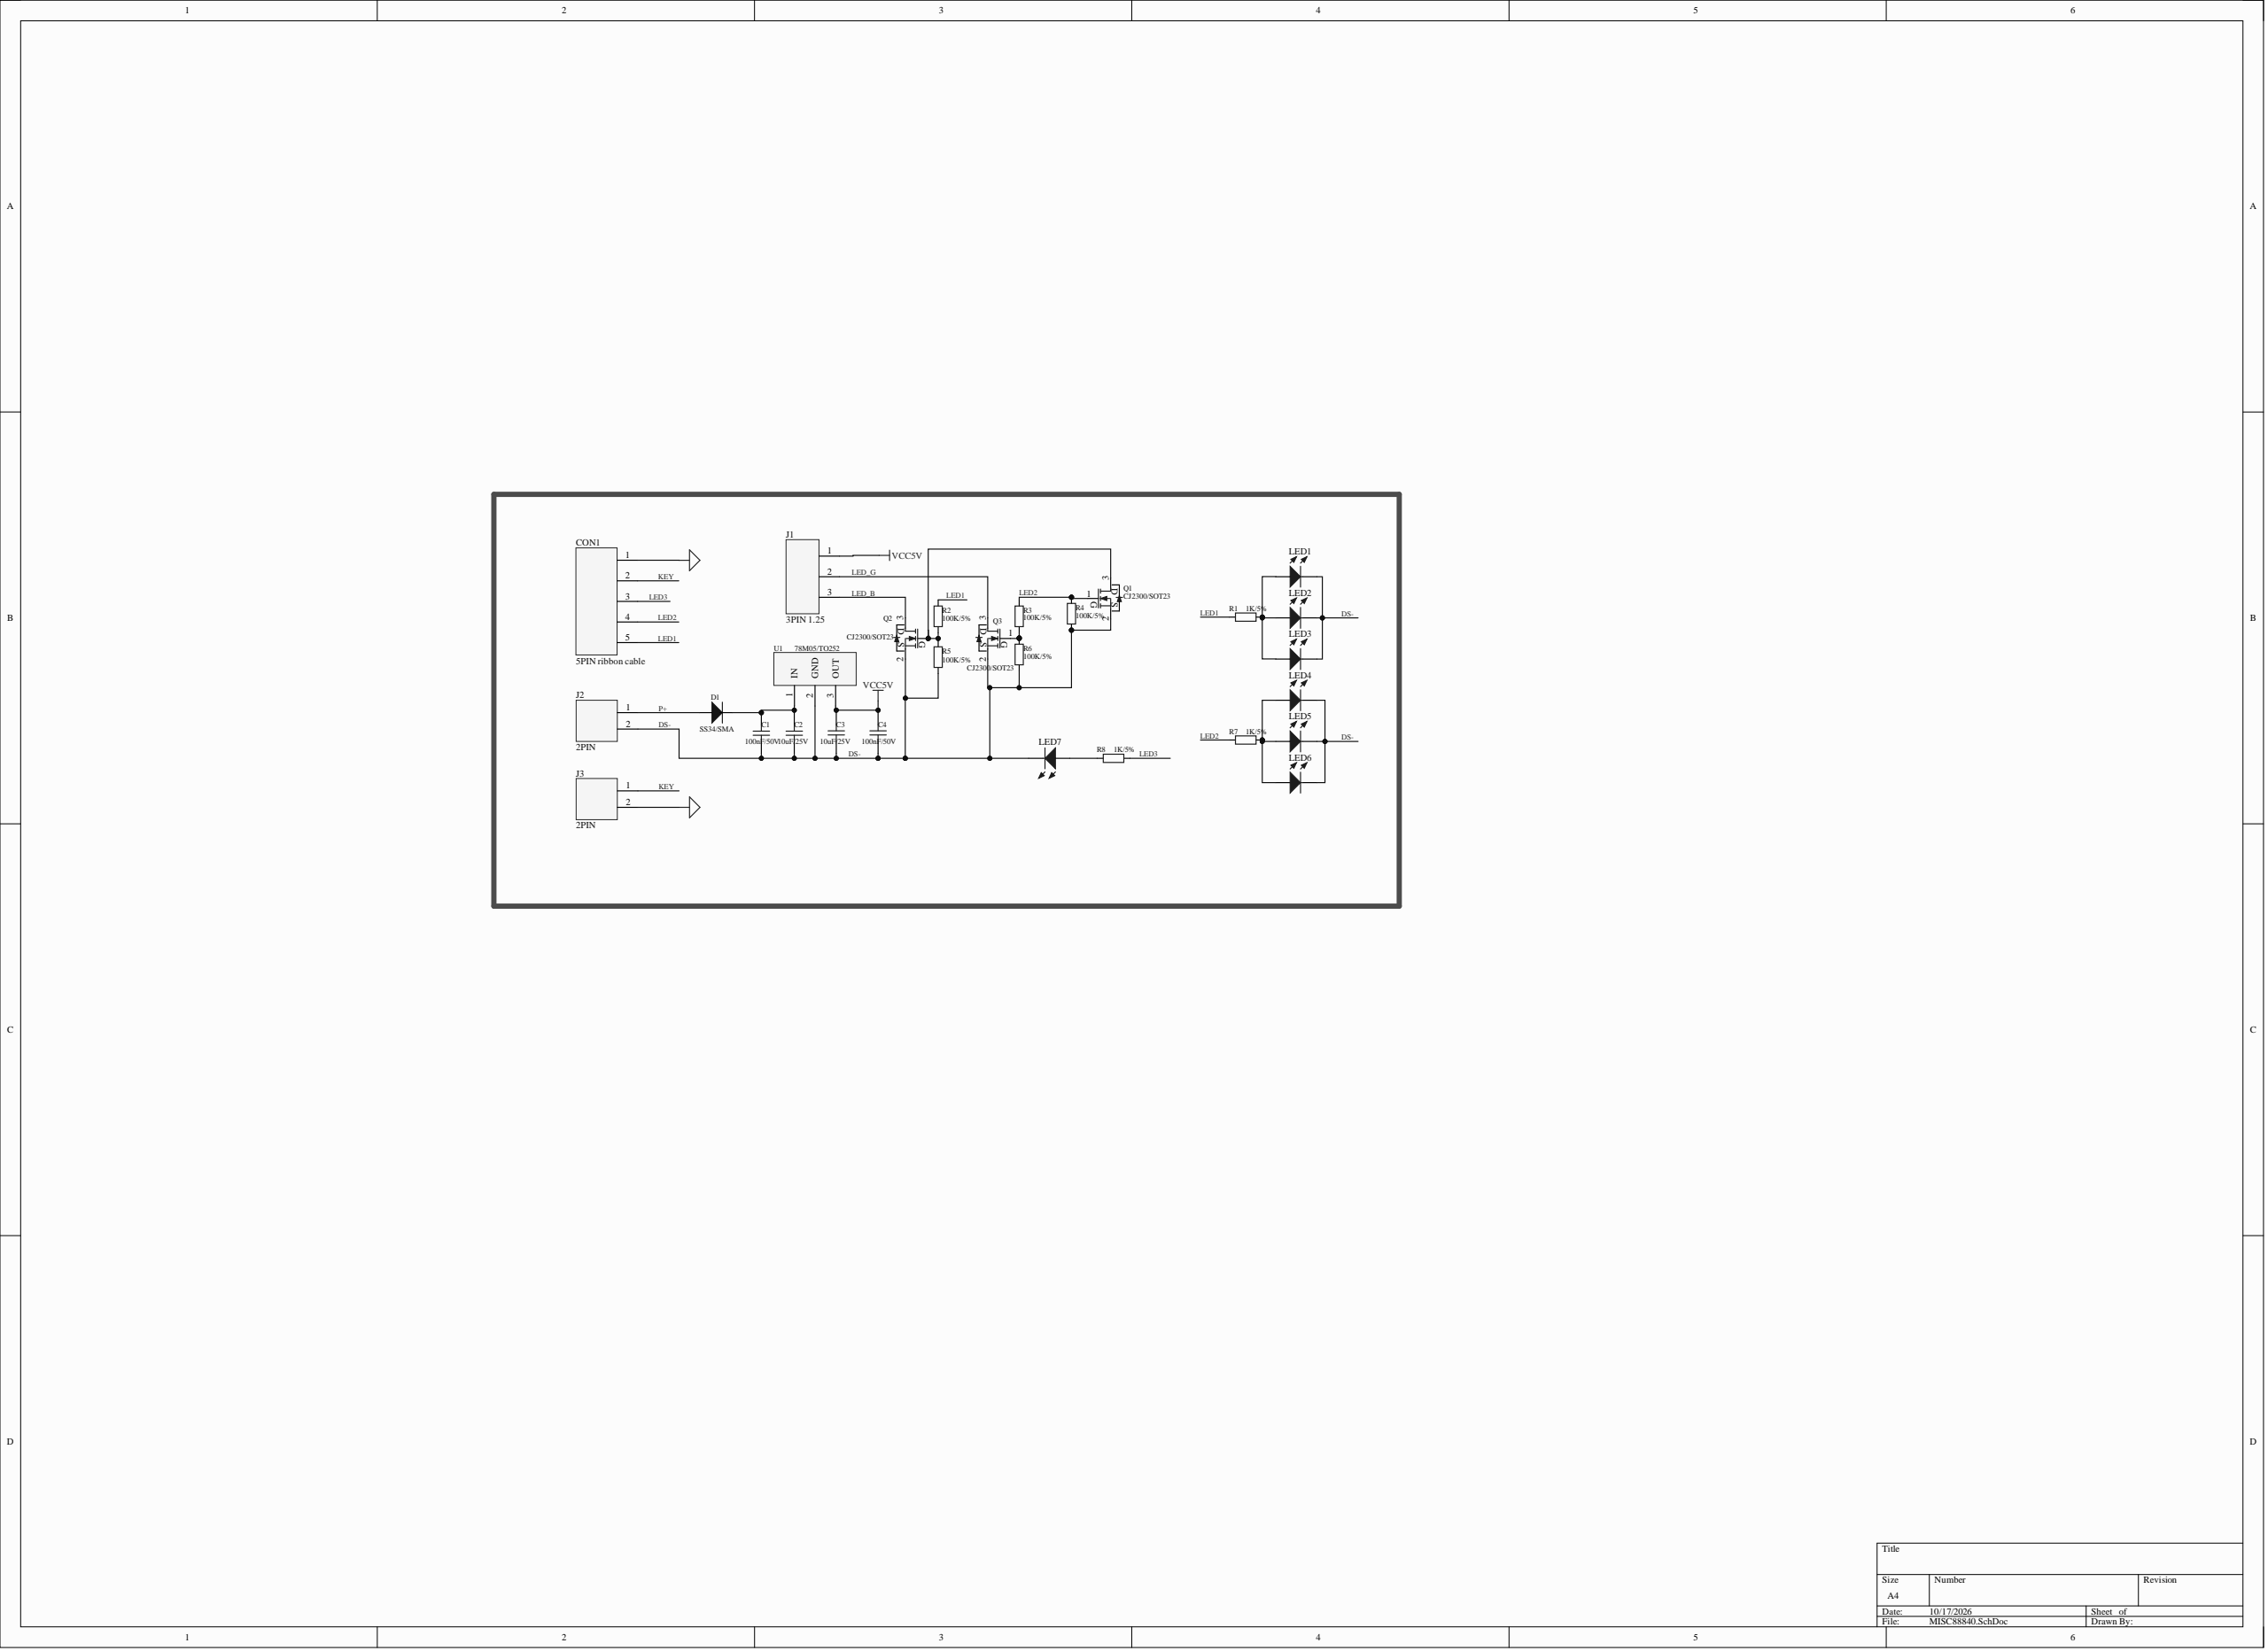Circuit board | Altium Designer | 28 parts | 16 nets
Bill of materials:
Comment,Description,Designator,Footprint,LibRef,Quantity
"100nF/50V","SMD capacitor","C1, C4","C0603A","C0603","2"
"10uF/25V","SMD capacitor","C2, C3","C0805A","C0805","2"
"5PIN ribbon cable","10PIN dual row","CON1","GH1.25-5PIN立贴带扣耐温260℃","5PIN","1"
"SS34/SMA","Fast recovery diode","D1","SOD323","T4","1"
"3PIN 1.25","DC socket 3PIN, 2.0 pitch","J1","GH1.25-3PIN立贴带扣耐温260℃","3PIN","1"
"2PIN","DC socket right angle 90°, 2.0 pitch","J2","HY2.0WT-2A/P 立贴带扣耐温260℃","2PIN","1"
"2PIN","DC socket right angle 90°, 2.0 pitch","J3","GH1.25-2PIN立贴带扣耐温260℃","2PIN","1"
"","SMD LED","LED1, LED2, LED3, LED4, LED5, LED6, LED7","LED0603A","LED 白发蓝","7"
"CJ2300/SOT23","Single N-channel MOSFET","Q1, Q2, Q3","SOT-23-3 MOS","MOS-N","3"
"1K/5%","SMD resistor","R1, R7, R8","R0603A","Res0603","3"
"100K/5%","SMD resistor","R2, R3, R4, R5, R6","R0603A","Res0603","5"
"78M05/TO252","SMD LDO","U1","TO-252-A","HT7533_SO89","1"
Netlist (Protel format):
[
C1
C0603A
100nF/50V



]
[
C2
C0805A
10uF/25V



]
[
C3
C0805A
10uF/25V



]
[
C4
C0603A
100nF/50V



]
[
CON1
GH1.25-5PIN立贴带扣耐温260℃
5PIN ribbon cable



]
[
D1
SOD323
SS34/SMA



]
[
J1
GH1.25-3PIN立贴带扣耐温260℃
3PIN 1.25



]
[
J2
HY2.0WT-2A/P 立贴带扣耐温260℃
2PIN



]
[
J3
GH1.25-2PIN立贴带扣耐温260℃
2PIN



]
[
LED1
LED0603A




]
[
LED2
LED0603A




]
[
LED3
LED0603A




]
[
LED4
LED0603A




]
[
LED5
LED0603A




]
[
LED6
LED0603A




]
[
LED7
LED0603A




]
[
Q1
SOT-23-3 MOS
CJ2300/SOT23



]
[
Q2
SOT-23-3 MOS
CJ2300/SOT23



]
[
Q3
SOT-23-3 MOS
CJ2300/SOT23



]
[
R1
R0603A
1K/5%



]
[
R2
R0603A
100K/5%



]
[
R3
R0603A
100K/5%



]
[
R4
R0603A
100K/5%



]
[
R5
R0603A
100K/5%



]
[
R6
R0603A
100K/5%



]
[
R7
R0603A
1K/5%



]
[
R8
R0603A
1K/5%



]
[
U1
TO-252-A
78M05/TO252



]
(
VCC5V
C3-2
C4-2
J1-1
U1-3
)
(
P+
D1-1
J2-1
)
(
NetQ3_1
Q3-1
R3-2
R6-2
)
(
NetQ1_3
Q1-3
Q2-1
R2-2
R5-2
)
(
NetLED7_1
LED7-1
R8-1
)
(
NetLED4_1
LED4-1
LED5-1
LED6-1
R7-2
)
(
NetLED1_1
LED1-1
LED2-1
LED3-1
R1-2
)
(
NetC1_2
C1-2
C2-2
D1-2
U1-1
)
(
LED_G
J1-2
Q3-3
)
(
LED_B
J1-3
Q2-3
)
(
LED3
CON1-3
R8-2
)
(
LED2
CON1-4
Q1-1
R3-1
R4-1
R7-1
)
(
LED1
CON1-5
R1-1
R2-1
)
(
KEY
CON1-2
J3-1
)
(
DS-
C1-1
C2-1
C3-1
C4-1
J2-2
LED1-2
LED2-2
LED3-2
LED4-2
LED5-2
LED6-2
LED7-2
Q1-2
Q2-2
Q3-2
R4-2
R5-1
R6-1
U1-2
)
(
B-
CON1-1
J3-2
)